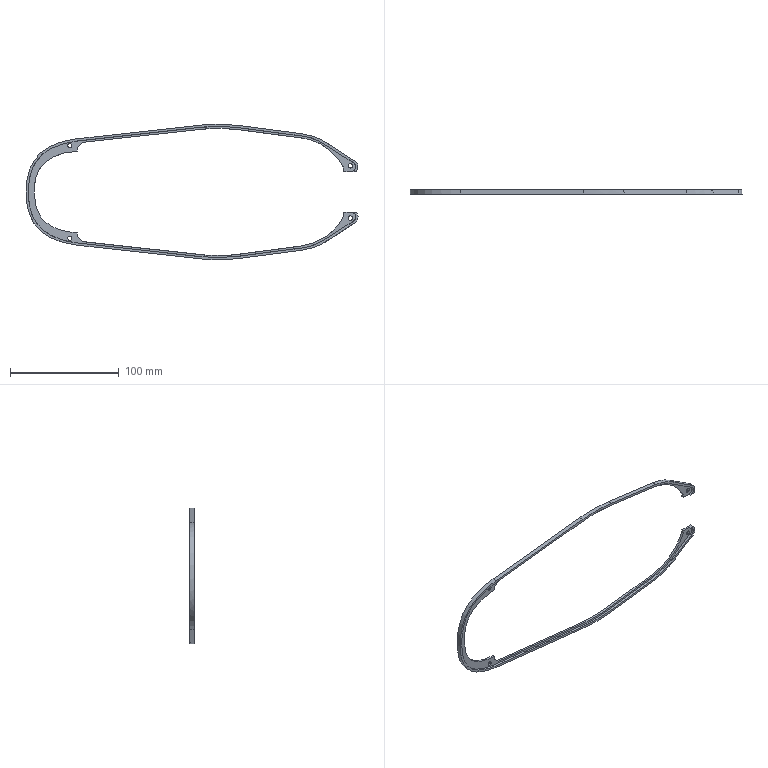Part | STEP file | 11-Cover21111 | 1 solid | 58 faces | box 305.265 x 4 x 124.613 mm | volume 9765 mm3 | plane 27 | spline 15 | cylinder 8 | cone 8 | commonest cylinder face diameters 4 x8